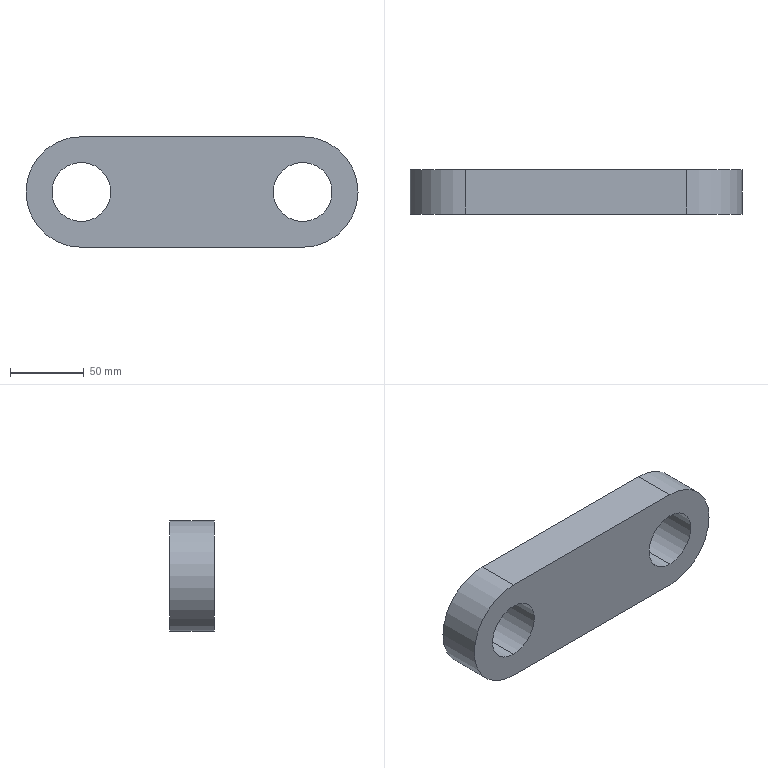Part | STEP file | LM-05-1223_default | 1 solid | 26 faces | box 225 x 30 x 75 mm | volume 393263 mm3 | cylinder 14 | cone 8 | plane 4 | commonest cylinder face diameters 5 x8 40 x4 75 x2